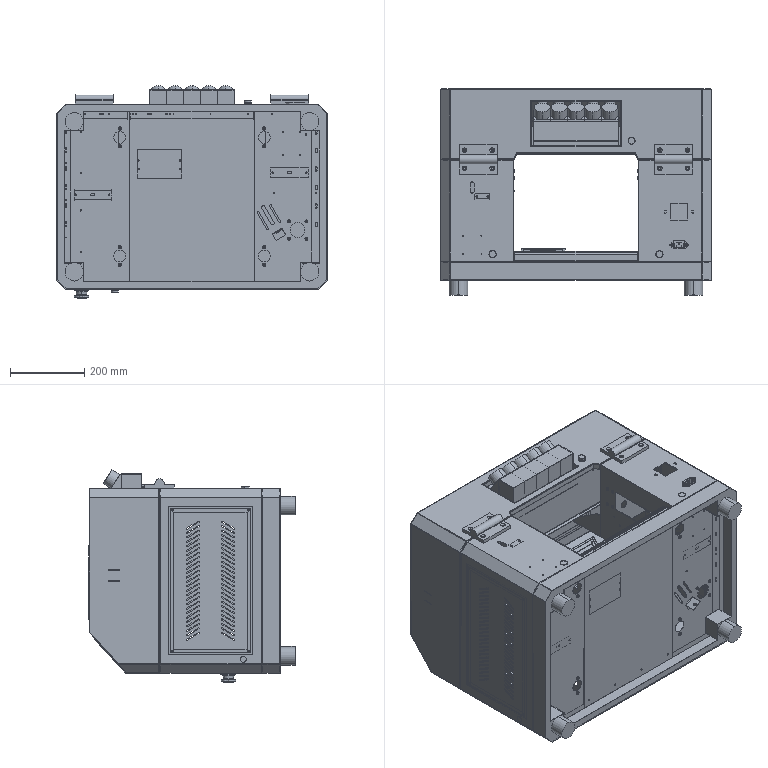Part | SolidWorks | 45 solids | 4748 faces | volume 6869314 mm3 | cylinder 2403 | plane 1700 | spline 515 | cone 66 | sphere 36 | torus 28 | commonest cylinder face diameters 3 x312 0.2 x239 40 x202 2.5 x200 0.5 x145 5 x142